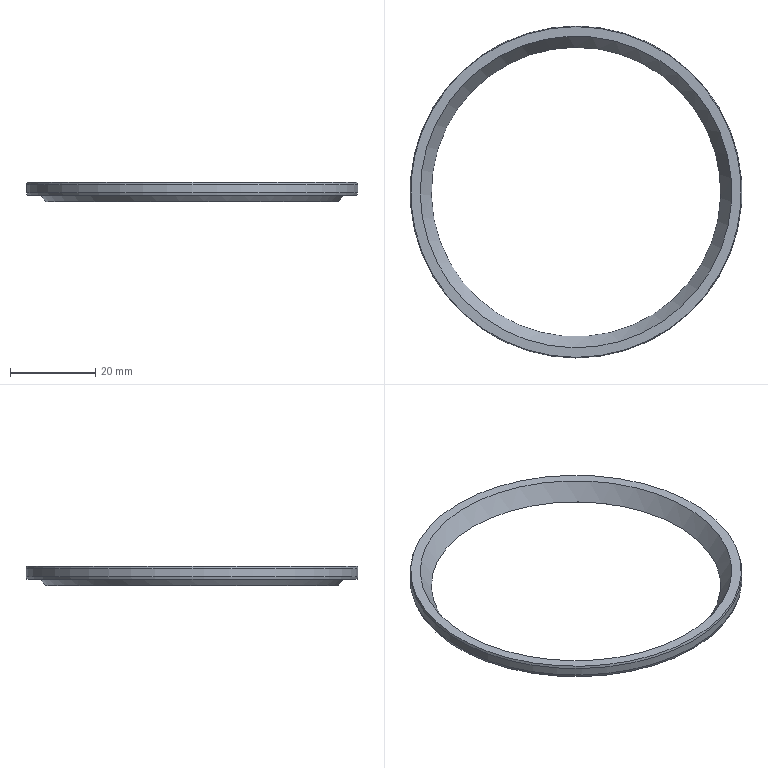Part | STEP file | 1 solid | 12 faces | box 78 x 78 x 4.5 mm | volume 2023 mm3 | cone 5 | plane 3 | cylinder 2 | torus 2 | commonest cylinder face diameters 75.4 x1 78 x1
STEP:
#1=CARTESIAN_POINT('',(33.645,-19.425,-11.25));
#2=VERTEX_POINT('',#1);
#3=CARTESIAN_POINT('',(0.,0.,-11.25));
#4=DIRECTION('',(0.,0.,1.));
#5=DIRECTION('',(0.866,0.5,0.));
#6=AXIS2_PLACEMENT_3D('',#3,#4,#5);
#7=CIRCLE('',#6,38.85);
#8=EDGE_CURVE('',#2,#2,#7,.T.);
#9=ORIENTED_EDGE('',*,*,#8,.T.);
#10=EDGE_LOOP('',(#9));
#11=FACE_BOUND('',#10,.T.);
#12=CARTESIAN_POINT('',(31.697,-18.3,-11.25));
#13=VERTEX_POINT('',#12);
#14=CARTESIAN_POINT('',(0.,0.,-11.25));
#15=DIRECTION('',(0.,0.,-1.));
#16=DIRECTION('',(0.,-1.,0.));
#17=AXIS2_PLACEMENT_3D('',#14,#15,#16);
#18=CIRCLE('',#17,36.6);
#19=EDGE_CURVE('',#13,#13,#18,.T.);
#20=ORIENTED_EDGE('',*,*,#19,.T.);
#21=EDGE_LOOP('',(#20));
#22=FACE_BOUND('',#21,.T.);
#23=CARTESIAN_POINT('',(0.,0.,-11.25));
#24=DIRECTION('',(0.,0.,-1.));
#25=DIRECTION('',(0.,-1.,0.));
#26=AXIS2_PLACEMENT_3D('',#23,#24,#25);
#27=PLANE('',#26);
#28=ADVANCED_FACE('',(#11,#22),#27,.F.);
#29=CARTESIAN_POINT('',(33.775,-19.5,-11.81));
#30=VERTEX_POINT('',#29);
#31=CARTESIAN_POINT('',(-33.775,19.5,-11.81));
#32=VERTEX_POINT('',#31);
#33=CARTESIAN_POINT('',(0.,0.,-11.81));
#34=DIRECTION('',(0.,0.,1.));
#35=DIRECTION('',(0.866,-0.5,0.));
#36=AXIS2_PLACEMENT_3D('',#33,#34,#35);
#37=CIRCLE('',#36,39.);
#38=EDGE_CURVE('',#30,#32,#37,.T.);
#39=ORIENTED_EDGE('',*,*,#38,.T.);
#40=CARTESIAN_POINT('',(0.,0.,-11.81));
#41=DIRECTION('',(0.,0.,1.));
#42=DIRECTION('',(-0.866,0.5,0.));
#43=AXIS2_PLACEMENT_3D('',#40,#41,#42);
#44=CIRCLE('',#43,39.);
#45=EDGE_CURVE('',#32,#30,#44,.T.);
#46=ORIENTED_EDGE('',*,*,#45,.T.);
#47=EDGE_LOOP('',(#39,#46));
#48=FACE_BOUND('',#47,.T.);
#49=ORIENTED_EDGE('',*,*,#8,.F.);
#50=EDGE_LOOP('',(#49));
#51=FACE_OUTER_BOUND('',#50,.T.);
#52=CARTESIAN_POINT('',(0.,0.,-11.53));
#53=DIRECTION('',(0.,0.,-1.));
#54=DIRECTION('',(0.866,-0.5,0.));
#55=AXIS2_PLACEMENT_3D('',#52,#53,#54);
#56=CONICAL_SURFACE('',#55,38.925,0.2617);
#57=ADVANCED_FACE('',(#48,#51),#56,.T.);
#58=ORIENTED_EDGE('',*,*,#45,.F.);
#59=ORIENTED_EDGE('',*,*,#38,.F.);
#60=EDGE_LOOP('',(#58,#59));
#61=FACE_BOUND('',#60,.T.);
#62=CARTESIAN_POINT('',(-33.775,19.5,-13.69));
#63=VERTEX_POINT('',#62);
#64=CARTESIAN_POINT('',(33.775,-19.5,-13.69));
#65=VERTEX_POINT('',#64);
#66=CARTESIAN_POINT('',(0.,0.,-13.69));
#67=DIRECTION('',(0.,0.,-1.));
#68=DIRECTION('',(-0.866,0.5,0.));
#69=AXIS2_PLACEMENT_3D('',#66,#67,#68);
#70=CIRCLE('',#69,39.);
#71=EDGE_CURVE('',#63,#65,#70,.T.);
#72=ORIENTED_EDGE('',*,*,#71,.F.);
#73=CARTESIAN_POINT('',(0.,0.,-13.69));
#74=DIRECTION('',(0.,0.,-1.));
#75=DIRECTION('',(0.866,-0.5,0.));
#76=AXIS2_PLACEMENT_3D('',#73,#74,#75);
#77=CIRCLE('',#76,39.);
#78=EDGE_CURVE('',#65,#63,#77,.T.);
#79=ORIENTED_EDGE('',*,*,#78,.F.);
#80=EDGE_LOOP('',(#72,#79));
#81=FACE_BOUND('',#80,.T.);
#82=CARTESIAN_POINT('',(0.,0.,-11.025));
#83=DIRECTION('',(0.,0.,1.));
#84=DIRECTION('',(0.866,-0.5,0.));
#85=AXIS2_PLACEMENT_3D('',#82,#83,#84);
#86=CYLINDRICAL_SURFACE('',#85,39.);
#87=ADVANCED_FACE('',(#61,#81),#86,.T.);
#88=ORIENTED_EDGE('',*,*,#78,.T.);
#89=ORIENTED_EDGE('',*,*,#71,.T.);
#90=EDGE_LOOP('',(#88,#89));
#91=FACE_BOUND('',#90,.T.);
#92=CARTESIAN_POINT('',(33.645,-19.425,-14.25));
#93=VERTEX_POINT('',#92);
#94=CARTESIAN_POINT('',(0.,0.,-14.25));
#95=DIRECTION('',(0.,0.,-1.));
#96=DIRECTION('',(0.,-1.,0.));
#97=AXIS2_PLACEMENT_3D('',#94,#95,#96);
#98=CIRCLE('',#97,38.85);
#99=EDGE_CURVE('',#93,#93,#98,.T.);
#100=ORIENTED_EDGE('',*,*,#99,.F.);
#101=EDGE_LOOP('',(#100));
#102=FACE_OUTER_BOUND('',#101,.T.);
#103=CARTESIAN_POINT('',(0.,0.,-13.97));
#104=DIRECTION('',(0.,0.,1.));
#105=DIRECTION('',(0.866,-0.5,0.));
#106=AXIS2_PLACEMENT_3D('',#103,#104,#105);
#107=CONICAL_SURFACE('',#106,38.925,0.2617);
#108=ADVANCED_FACE('',(#91,#102),#107,.T.);
#109=ORIENTED_EDGE('',*,*,#99,.T.);
#110=EDGE_LOOP('',(#109));
#111=FACE_BOUND('',#110,.T.);
#112=CARTESIAN_POINT('',(-32.649,18.85,-14.25));
#113=VERTEX_POINT('',#112);
#114=CARTESIAN_POINT('',(0.,0.,-14.25));
#115=DIRECTION('',(0.,0.,1.));
#116=DIRECTION('',(0.866,-0.5,0.));
#117=AXIS2_PLACEMENT_3D('',#114,#115,#116);
#118=CIRCLE('',#117,37.7);
#119=EDGE_CURVE('',#113,#113,#118,.T.);
#120=ORIENTED_EDGE('',*,*,#119,.T.);
#121=EDGE_LOOP('',(#120));
#122=FACE_BOUND('',#121,.T.);
#123=CARTESIAN_POINT('',(0.,0.,-14.25));
#124=DIRECTION('',(0.,0.,-1.));
#125=DIRECTION('',(0.,-1.,0.));
#126=AXIS2_PLACEMENT_3D('',#123,#124,#125);
#127=PLANE('',#126);
#128=ADVANCED_FACE('',(#111,#122),#127,.T.);
#129=CARTESIAN_POINT('',(-32.649,18.85,-13.05));
#130=VERTEX_POINT('',#129);
#131=CARTESIAN_POINT('',(-32.649,18.85,-13.05));
#132=CARTESIAN_POINT('',(-32.254,19.534,-13.05));
#133=CARTESIAN_POINT('',(-31.422,20.877,-13.05));
#134=CARTESIAN_POINT('',(-30.048,22.809,-13.05));
#135=CARTESIAN_POINT('',(-28.557,24.651,-13.05));
#136=CARTESIAN_POINT('',(-26.952,26.396,-13.05));
#137=CARTESIAN_POINT('',(-25.241,28.036,-13.05));
#138=CARTESIAN_POINT('',(-23.431,29.566,-13.05));
#139=CARTESIAN_POINT('',(-21.528,30.979,-13.05));
#140=CARTESIAN_POINT('',(-19.54,32.27,-13.05));
#141=CARTESIAN_POINT('',(-17.475,33.433,-13.05));
#142=CARTESIAN_POINT('',(-15.341,34.465,-13.05));
#143=CARTESIAN_POINT('',(-13.146,35.36,-13.05));
#144=CARTESIAN_POINT('',(-10.899,36.116,-13.05));
#145=CARTESIAN_POINT('',(-8.61,36.729,-13.05));
#146=CARTESIAN_POINT('',(-6.286,37.197,-13.05));
#147=CARTESIAN_POINT('',(-3.938,37.519,-13.05));
#148=CARTESIAN_POINT('',(-1.574,37.692,-13.05));
#149=CARTESIAN_POINT('',(0.7965,37.716,-13.05));
#150=CARTESIAN_POINT('',(3.163,37.592,-13.05));
#151=CARTESIAN_POINT('',(5.518,37.319,-13.05));
#152=CARTESIAN_POINT('',(7.851,36.899,-13.05));
#153=CARTESIAN_POINT('',(10.153,36.333,-13.05));
#154=CARTESIAN_POINT('',(12.414,35.624,-13.05));
#155=CARTESIAN_POINT('',(14.627,34.774,-13.05));
#156=CARTESIAN_POINT('',(16.782,33.787,-13.05));
#157=CARTESIAN_POINT('',(18.871,32.666,-13.05));
#158=CARTESIAN_POINT('',(20.885,31.416,-13.05));
#159=CARTESIAN_POINT('',(22.817,30.043,-13.05));
#160=CARTESIAN_POINT('',(24.658,28.551,-13.05));
#161=CARTESIAN_POINT('',(26.402,26.946,-13.05));
#162=CARTESIAN_POINT('',(28.043,25.234,-13.05));
#163=CARTESIAN_POINT('',(29.572,23.424,-13.05));
#164=CARTESIAN_POINT('',(30.985,21.52,-13.05));
#165=CARTESIAN_POINT('',(32.275,19.532,-13.05));
#166=CARTESIAN_POINT('',(33.438,17.466,-13.05));
#167=CARTESIAN_POINT('',(34.469,15.332,-13.05));
#168=CARTESIAN_POINT('',(35.364,13.137,-13.05));
#169=CARTESIAN_POINT('',(36.119,10.89,-13.05));
#170=CARTESIAN_POINT('',(36.731,8.601,-13.05));
#171=CARTESIAN_POINT('',(37.199,6.277,-13.05));
#172=CARTESIAN_POINT('',(37.52,3.928,-13.05));
#173=CARTESIAN_POINT('',(37.692,1.564,-13.05));
#174=CARTESIAN_POINT('',(37.716,-0.8059,-13.05));
#175=CARTESIAN_POINT('',(37.591,-3.173,-13.05));
#176=CARTESIAN_POINT('',(37.318,-5.527,-13.05));
#177=CARTESIAN_POINT('',(36.897,-7.86,-13.05));
#178=CARTESIAN_POINT('',(36.33,-10.162,-13.05));
#179=CARTESIAN_POINT('',(35.621,-12.423,-13.05));
#180=CARTESIAN_POINT('',(34.77,-14.636,-13.05));
#181=CARTESIAN_POINT('',(33.785,-16.785,-13.05));
#182=CARTESIAN_POINT('',(33.041,-18.172,-13.05));
#183=CARTESIAN_POINT('',(32.649,-18.85,-13.05));
#184=CARTESIAN_POINT('',(32.254,-19.534,-13.05));
#185=CARTESIAN_POINT('',(31.422,-20.877,-13.05));
#186=CARTESIAN_POINT('',(30.048,-22.809,-13.05));
#187=CARTESIAN_POINT('',(28.557,-24.651,-13.05));
#188=CARTESIAN_POINT('',(26.952,-26.396,-13.05));
#189=CARTESIAN_POINT('',(25.241,-28.036,-13.05));
#190=CARTESIAN_POINT('',(23.431,-29.566,-13.05));
#191=CARTESIAN_POINT('',(21.528,-30.979,-13.05));
#192=CARTESIAN_POINT('',(19.54,-32.27,-13.05));
#193=CARTESIAN_POINT('',(17.475,-33.433,-13.05));
#194=CARTESIAN_POINT('',(15.341,-34.465,-13.05));
#195=CARTESIAN_POINT('',(13.146,-35.36,-13.05));
#196=CARTESIAN_POINT('',(10.899,-36.116,-13.05));
#197=CARTESIAN_POINT('',(8.61,-36.729,-13.05));
#198=CARTESIAN_POINT('',(6.286,-37.197,-13.05));
#199=CARTESIAN_POINT('',(3.938,-37.519,-13.05));
#200=CARTESIAN_POINT('',(1.574,-37.692,-13.05));
#201=CARTESIAN_POINT('',(-0.7965,-37.716,-13.05));
#202=CARTESIAN_POINT('',(-3.163,-37.592,-13.05));
#203=CARTESIAN_POINT('',(-5.518,-37.319,-13.05));
#204=CARTESIAN_POINT('',(-7.851,-36.899,-13.05));
#205=CARTESIAN_POINT('',(-10.153,-36.333,-13.05));
#206=CARTESIAN_POINT('',(-12.414,-35.624,-13.05));
#207=CARTESIAN_POINT('',(-14.627,-34.774,-13.05));
#208=CARTESIAN_POINT('',(-16.782,-33.787,-13.05));
#209=CARTESIAN_POINT('',(-18.871,-32.666,-13.05));
#210=CARTESIAN_POINT('',(-20.885,-31.416,-13.05));
#211=CARTESIAN_POINT('',(-22.817,-30.043,-13.05));
#212=CARTESIAN_POINT('',(-24.658,-28.551,-13.05));
#213=CARTESIAN_POINT('',(-26.402,-26.946,-13.05));
#214=CARTESIAN_POINT('',(-28.043,-25.234,-13.05));
#215=CARTESIAN_POINT('',(-29.572,-23.424,-13.05));
#216=CARTESIAN_POINT('',(-30.985,-21.52,-13.05));
#217=CARTESIAN_POINT('',(-32.275,-19.532,-13.05));
#218=CARTESIAN_POINT('',(-33.438,-17.466,-13.05));
#219=CARTESIAN_POINT('',(-34.469,-15.332,-13.05));
#220=CARTESIAN_POINT('',(-35.364,-13.137,-13.05));
#221=CARTESIAN_POINT('',(-36.119,-10.89,-13.05));
#222=CARTESIAN_POINT('',(-36.731,-8.601,-13.05));
#223=CARTESIAN_POINT('',(-37.199,-6.277,-13.05));
#224=CARTESIAN_POINT('',(-37.52,-3.928,-13.05));
#225=CARTESIAN_POINT('',(-37.692,-1.564,-13.05));
#226=CARTESIAN_POINT('',(-37.716,0.8059,-13.05));
#227=CARTESIAN_POINT('',(-37.591,3.173,-13.05));
#228=CARTESIAN_POINT('',(-37.318,5.527,-13.05));
#229=CARTESIAN_POINT('',(-36.897,7.86,-13.05));
#230=CARTESIAN_POINT('',(-36.33,10.162,-13.05));
#231=CARTESIAN_POINT('',(-35.621,12.423,-13.05));
#232=CARTESIAN_POINT('',(-34.77,14.636,-13.05));
#233=CARTESIAN_POINT('',(-33.785,16.785,-13.05));
#234=CARTESIAN_POINT('',(-33.041,18.172,-13.05));
#235=CARTESIAN_POINT('',(-32.649,18.85,-13.05));
#236=B_SPLINE_CURVE_WITH_KNOTS('',3,(#131,#132,#133,#134,#135,#136,#137,#138,#139,#140,#141,#142,#143,#144,#145,#146,#147,#148,#149,#150,#151,#152,#153,#154,#155,#156,#157,#158,#159,#160,#161,#162,#163,#164,#165,#166,#167,#168,#169,#170,#171,#172,#173,#174,#175,#176,#177,#178,#179,#180,#181,#182,#183,#184,#185,#186,#187,#188,#189,#190,#191,#192,#193,#194,#195,#196,#197,#198,#199,#200,#201,#202,#203,#204,#205,#206,#207,#208,#209,#210,#211,#212,#213,#214,#215,#216,#217,#218,#219,#220,#221,#222,#223,#224,#225,#226,#227,#228,#229,#230,#231,#232,#233,#234,#235),.UNSPECIFIED.,.T.,.F.,(4,1,1,1,1,1,1,1,1,1,1,1,1,1,1,1,1,1,1,1,1,1,1,1,1,1,1,1,1,1,1,1,1,1,1,1,1,1,1,1,1,1,1,1,1,1,1,1,1,1,3,1,1,1,1,1,1,1,1,1,1,1,1,1,1,1,1,1,1,1,1,1,1,1,1,1,1,1,1,1,1,1,1,1,1,1,1,1,1,1,1,1,1,1,1,1,1,1,1,1,4),(0.,0.01,0.02,0.03,0.04001,0.05001,0.06001,0.07001,0.08001,0.09001,0.1,0.11,0.12,0.13,0.14,0.15,0.16,0.17,0.18,0.19,0.2,0.21,0.22,0.23,0.24,0.25,0.26,0.27,0.28,0.29,0.3,0.31,0.3201,0.3301,0.3401,0.3501,0.3601,0.3701,0.3801,0.3901,0.4001,0.4101,0.4201,0.4301,0.4401,0.4501,0.4601,0.4701,0.4801,0.4901,0.5,0.51,0.52,0.53,0.54,0.55,0.56,0.57,0.58,0.59,0.6,0.61,0.62,0.63,0.64,0.65,0.66,0.67,0.68,0.69,0.7,0.71,0.72,0.73,0.74,0.75,0.76,0.77,0.78,0.79,0.8,0.81,0.8201,0.8301,0.8401,0.8501,0.8601,0.8701,0.8801,0.8901,0.9001,0.9101,0.9201,0.9301,0.9401,0.9501,0.9601,0.9701,0.9801,0.9901,1.),.UNSPECIFIED.);
#237=EDGE_CURVE('',#130,#130,#236,.T.);
#238=ORIENTED_EDGE('',*,*,#237,.F.);
#239=EDGE_LOOP('',(#238));
#240=FACE_OUTER_BOUND('',#239,.T.);
#241=ORIENTED_EDGE('',*,*,#119,.F.);
#242=EDGE_LOOP('',(#241));
#243=FACE_OUTER_BOUND('',#242,.T.);
#244=CARTESIAN_POINT('',(0.,0.,-11.025));
#245=DIRECTION('',(0.,0.,1.));
#246=DIRECTION('',(0.866,-0.5,0.));
#247=AXIS2_PLACEMENT_3D('',#244,#245,#246);
#248=CYLINDRICAL_SURFACE('',#247,37.7);
#249=ADVANCED_FACE('',(#240,#243),#248,.F.);
#250=CARTESIAN_POINT('',(-32.389,18.7,-12.75));
#251=VERTEX_POINT('',#250);
#252=CARTESIAN_POINT('',(0.,0.,-12.75));
#253=DIRECTION('',(0.,0.,-1.));
#254=DIRECTION('',(0.866,-0.5,0.));
#255=AXIS2_PLACEMENT_3D('',#252,#253,#254);
#256=CIRCLE('',#255,37.4);
#257=EDGE_CURVE('',#251,#251,#256,.T.);
#258=ORIENTED_EDGE('',*,*,#257,.F.);
#259=EDGE_LOOP('',(#258));
#260=FACE_OUTER_BOUND('',#259,.T.);
#261=ORIENTED_EDGE('',*,*,#237,.T.);
#262=EDGE_LOOP('',(#261));
#263=FACE_OUTER_BOUND('',#262,.T.);
#264=CARTESIAN_POINT('',(0.,0.,-13.05));
#265=DIRECTION('',(0.,0.,-1.));
#266=DIRECTION('',(0.866,-0.5,0.));
#267=AXIS2_PLACEMENT_3D('',#264,#265,#266);
#268=TOROIDAL_SURFACE('',#267,37.4,0.3);
#269=ADVANCED_FACE('',(#260,#263),#268,.F.);
#270=ORIENTED_EDGE('',*,*,#257,.T.);
#271=EDGE_LOOP('',(#270));
#272=FACE_BOUND('',#271,.T.);
#273=CARTESIAN_POINT('',(-32.008,18.48,-12.75));
#274=VERTEX_POINT('',#273);
#275=CARTESIAN_POINT('',(0.,0.,-12.75));
#276=DIRECTION('',(0.,0.,1.));
#277=DIRECTION('',(0.866,-0.5,0.));
#278=AXIS2_PLACEMENT_3D('',#275,#276,#277);
#279=CIRCLE('',#278,36.959);
#280=EDGE_CURVE('',#274,#274,#279,.T.);
#281=ORIENTED_EDGE('',*,*,#280,.T.);
#282=EDGE_LOOP('',(#281));
#283=FACE_BOUND('',#282,.T.);
#284=CARTESIAN_POINT('',(0.,0.,-12.75));
#285=DIRECTION('',(0.,0.,-1.));
#286=DIRECTION('',(0.,-1.,0.));
#287=AXIS2_PLACEMENT_3D('',#284,#285,#286);
#288=PLANE('',#287);
#289=ADVANCED_FACE('',(#272,#283),#288,.T.);
#290=CARTESIAN_POINT('',(31.804,-18.362,-12.863));
#291=VERTEX_POINT('',#290);
#292=CARTESIAN_POINT('',(-31.804,18.362,-12.863));
#293=VERTEX_POINT('',#292);
#294=CARTESIAN_POINT('',(0.,0.,-12.863));
#295=DIRECTION('',(0.,0.,1.));
#296=DIRECTION('',(0.866,-0.5,0.));
#297=AXIS2_PLACEMENT_3D('',#294,#295,#296);
#298=CIRCLE('',#297,36.725);
#299=EDGE_CURVE('',#291,#293,#298,.T.);
#300=ORIENTED_EDGE('',*,*,#299,.T.);
#301=CARTESIAN_POINT('',(0.,0.,-12.863));
#302=DIRECTION('',(0.,0.,1.));
#303=DIRECTION('',(-0.866,0.5,0.));
#304=AXIS2_PLACEMENT_3D('',#301,#302,#303);
#305=CIRCLE('',#304,36.725);
#306=EDGE_CURVE('',#293,#291,#305,.T.);
#307=ORIENTED_EDGE('',*,*,#306,.T.);
#308=EDGE_LOOP('',(#300,#307));
#309=FACE_BOUND('',#308,.T.);
#310=ORIENTED_EDGE('',*,*,#280,.F.);
#311=EDGE_LOOP('',(#310));
#312=FACE_OUTER_BOUND('',#311,.T.);
#313=CARTESIAN_POINT('',(0.,0.,-13.05));
#314=DIRECTION('',(0.,0.,-1.));
#315=DIRECTION('',(0.866,-0.5,0.));
#316=AXIS2_PLACEMENT_3D('',#313,#314,#315);
#317=TOROIDAL_SURFACE('',#316,36.959,0.3);
#318=ADVANCED_FACE('',(#309,#312),#317,.F.);
#319=ORIENTED_EDGE('',*,*,#306,.F.);
#320=ORIENTED_EDGE('',*,*,#299,.F.);
#321=EDGE_LOOP('',(#319,#320));
#322=FACE_BOUND('',#321,.T.);
#323=CARTESIAN_POINT('',(29.814,-17.213,-15.75));
#324=VERTEX_POINT('',#323);
#325=CARTESIAN_POINT('',(29.814,-17.213,-15.75));
#326=CARTESIAN_POINT('',(29.453,-17.838,-15.75));
#327=CARTESIAN_POINT('',(28.693,-19.064,-15.75));
#328=CARTESIAN_POINT('',(27.439,-20.828,-15.75));
#329=CARTESIAN_POINT('',(26.077,-22.51,-15.75));
#330=CARTESIAN_POINT('',(24.612,-24.104,-15.75));
#331=CARTESIAN_POINT('',(23.05,-25.602,-15.75));
#332=CARTESIAN_POINT('',(21.396,-26.999,-15.75));
#333=CARTESIAN_POINT('',(19.658,-28.289,-15.75));
#334=CARTESIAN_POINT('',(17.843,-29.468,-15.75));
#335=CARTESIAN_POINT('',(15.957,-30.53,-15.75));
#336=CARTESIAN_POINT('',(14.008,-31.472,-15.75));
#337=CARTESIAN_POINT('',(12.004,-32.29,-15.75));
#338=CARTESIAN_POINT('',(9.953,-32.98,-15.75));
#339=CARTESIAN_POINT('',(7.862,-33.54,-15.75));
#340=CARTESIAN_POINT('',(5.74,-33.967,-15.75));
#341=CARTESIAN_POINT('',(3.596,-34.261,-15.75));
#342=CARTESIAN_POINT('',(1.437,-34.419,-15.75));
#343=CARTESIAN_POINT('',(-0.7273,-34.441,-15.75));
#344=CARTESIAN_POINT('',(-2.889,-34.328,-15.75));
#345=CARTESIAN_POINT('',(-5.039,-34.078,-15.75));
#346=CARTESIAN_POINT('',(-7.169,-33.695,-15.75));
#347=CARTESIAN_POINT('',(-9.271,-33.178,-15.75));
#348=CARTESIAN_POINT('',(-11.336,-32.53,-15.75));
#349=CARTESIAN_POINT('',(-13.357,-31.754,-15.75));
#350=CARTESIAN_POINT('',(-15.325,-30.853,-15.75));
#351=CARTESIAN_POINT('',(-17.232,-29.829,-15.75));
#352=CARTESIAN_POINT('',(-19.071,-28.688,-15.75));
#353=CARTESIAN_POINT('',(-20.835,-27.434,-15.75));
#354=CARTESIAN_POINT('',(-22.517,-26.071,-15.75));
#355=CARTESIAN_POINT('',(-24.11,-24.606,-15.75));
#356=CARTESIAN_POINT('',(-25.607,-23.043,-15.75));
#357=CARTESIAN_POINT('',(-27.004,-21.389,-15.75));
#358=CARTESIAN_POINT('',(-28.294,-19.651,-15.75));
#359=CARTESIAN_POINT('',(-29.472,-17.836,-15.75));
#360=CARTESIAN_POINT('',(-30.534,-15.95,-15.75));
#361=CARTESIAN_POINT('',(-31.476,-14.001,-15.75));
#362=CARTESIAN_POINT('',(-32.293,-11.996,-15.75));
#363=CARTESIAN_POINT('',(-32.982,-9.945,-15.75));
#364=CARTESIAN_POINT('',(-33.542,-7.854,-15.75));
#365=CARTESIAN_POINT('',(-33.969,-5.732,-15.75));
#366=CARTESIAN_POINT('',(-34.262,-3.587,-15.75));
#367=CARTESIAN_POINT('',(-34.419,-1.428,-15.75));
#368=CARTESIAN_POINT('',(-34.441,0.7359,-15.75));
#369=CARTESIAN_POINT('',(-34.327,2.897,-15.75));
#370=CARTESIAN_POINT('',(-34.077,5.047,-15.75));
#371=CARTESIAN_POINT('',(-33.693,7.177,-15.75));
#372=CARTESIAN_POINT('',(-33.176,9.279,-15.75));
#373=CARTESIAN_POINT('',(-32.527,11.344,-15.75));
#374=CARTESIAN_POINT('',(-31.751,13.365,-15.75));
#375=CARTESIAN_POINT('',(-30.851,15.327,-15.75));
#376=CARTESIAN_POINT('',(-30.172,16.594,-15.75));
#377=CARTESIAN_POINT('',(-29.814,17.213,-15.75));
#378=CARTESIAN_POINT('',(-29.453,17.838,-15.75));
#379=CARTESIAN_POINT('',(-28.693,19.064,-15.75));
#380=CARTESIAN_POINT('',(-27.439,20.828,-15.75));
#381=CARTESIAN_POINT('',(-26.077,22.51,-15.75));
#382=CARTESIAN_POINT('',(-24.612,24.104,-15.75));
#383=CARTESIAN_POINT('',(-23.05,25.602,-15.75));
#384=CARTESIAN_POINT('',(-21.396,26.999,-15.75));
#385=CARTESIAN_POINT('',(-19.658,28.289,-15.75));
#386=CARTESIAN_POINT('',(-17.843,29.468,-15.75));
#387=CARTESIAN_POINT('',(-15.957,30.53,-15.75));
#388=CARTESIAN_POINT('',(-14.008,31.472,-15.75));
#389=CARTESIAN_POINT('',(-12.004,32.29,-15.75));
#390=CARTESIAN_POINT('',(-9.953,32.98,-15.75));
#391=CARTESIAN_POINT('',(-7.862,33.54,-15.75));
#392=CARTESIAN_POINT('',(-5.74,33.967,-15.75));
#393=CARTESIAN_POINT('',(-3.596,34.261,-15.75));
#394=CARTESIAN_POINT('',(-1.437,34.419,-15.75));
#395=CARTESIAN_POINT('',(0.7273,34.441,-15.75));
#396=CARTESIAN_POINT('',(2.889,34.328,-15.75));
#397=CARTESIAN_POINT('',(5.039,34.078,-15.75));
#398=CARTESIAN_POINT('',(7.169,33.695,-15.75));
#399=CARTESIAN_POINT('',(9.271,33.178,-15.75));
#400=CARTESIAN_POINT('',(11.336,32.53,-15.75));
#401=CARTESIAN_POINT('',(13.357,31.754,-15.75));
#402=CARTESIAN_POINT('',(15.325,30.853,-15.75));
#403=CARTESIAN_POINT('',(17.232,29.829,-15.75));
#404=CARTESIAN_POINT('',(19.071,28.688,-15.75));
#405=CARTESIAN_POINT('',(20.835,27.434,-15.75));
#406=CARTESIAN_POINT('',(22.517,26.071,-15.75));
#407=CARTESIAN_POINT('',(24.11,24.606,-15.75));
#408=CARTESIAN_POINT('',(25.607,23.043,-15.75));
#409=CARTESIAN_POINT('',(27.004,21.389,-15.75));
#410=CARTESIAN_POINT('',(28.294,19.651,-15.75));
#411=CARTESIAN_POINT('',(29.472,17.836,-15.75));
#412=CARTESIAN_POINT('',(30.534,15.95,-15.75));
#413=CARTESIAN_POINT('',(31.476,14.001,-15.75));
#414=CARTESIAN_POINT('',(32.293,11.996,-15.75));
#415=CARTESIAN_POINT('',(32.982,9.945,-15.75));
#416=CARTESIAN_POINT('',(33.542,7.854,-15.75));
#417=CARTESIAN_POINT('',(33.969,5.732,-15.75));
#418=CARTESIAN_POINT('',(34.262,3.587,-15.75));
#419=CARTESIAN_POINT('',(34.419,1.428,-15.75));
#420=CARTESIAN_POINT('',(34.441,-0.7359,-15.75));
#421=CARTESIAN_POINT('',(34.327,-2.897,-15.75));
#422=CARTESIAN_POINT('',(34.077,-5.047,-15.75));
#423=CARTESIAN_POINT('',(33.693,-7.177,-15.75));
#424=CARTESIAN_POINT('',(33.176,-9.279,-15.75));
#425=CARTESIAN_POINT('',(32.527,-11.344,-15.75));
#426=CARTESIAN_POINT('',(31.751,-13.365,-15.75));
#427=CARTESIAN_POINT('',(30.851,-15.327,-15.75));
#428=CARTESIAN_POINT('',(30.172,-16.594,-15.75));
#429=CARTESIAN_POINT('',(29.814,-17.213,-15.75));
#430=B_SPLINE_CURVE_WITH_KNOTS('',3,(#325,#326,#327,#328,#329,#330,#331,#332,#333,#334,#335,#336,#337,#338,#339,#340,#341,#342,#343,#344,#345,#346,#347,#348,#349,#350,#351,#352,#353,#354,#355,#356,#357,#358,#359,#360,#361,#362,#363,#364,#365,#366,#367,#368,#369,#370,#371,#372,#373,#374,#375,#376,#377,#378,#379,#380,#381,#382,#383,#384,#385,#386,#387,#388,#389,#390,#391,#392,#393,#394,#395,#396,#397,#398,#399,#400,#401,#402,#403,#404,#405,#406,#407,#408,#409,#410,#411,#412,#413,#414,#415,#416,#417,#418,#419,#420,#421,#422,#423,#424,#425,#426,#427,#428,#429),.UNSPECIFIED.,.T.,.F.,(4,1,1,1,1,1,1,1,1,1,1,1,1,1,1,1,1,1,1,1,1,1,1,1,1,1,1,1,1,1,1,1,1,1,1,1,1,1,1,1,1,1,1,1,1,1,1,1,1,1,3,1,1,1,1,1,1,1,1,1,1,1,1,1,1,1,1,1,1,1,1,1,1,1,1,1,1,1,1,1,1,1,1,1,1,1,1,1,1,1,1,1,1,1,1,1,1,1,1,1,4),(0.,0.01,0.02,0.03,0.04001,0.05001,0.06001,0.07001,0.08001,0.09001,0.1,0.11,0.12,0.13,0.14,0.15,0.16,0.17,0.18,0.19,0.2,0.21,0.22,0.23,0.24,0.25,0.26,0.27,0.28,0.29,0.3,0.31,0.3201,0.3301,0.3401,0.3501,0.3601,0.3701,0.3801,0.3901,0.4001,0.4101,0.4201,0.4301,0.4401,0.4501,0.4601,0.4701,0.4801,0.4901,0.5,0.51,0.52,0.53,0.54,0.55,0.56,0.57,0.58,0.59,0.6,0.61,0.62,0.63,0.64,0.65,0.66,0.67,0.68,0.69,0.7,0.71,0.72,0.73,0.74,0.75,0.76,0.77,0.78,0.79,0.8,0.81,0.8201,0.8301,0.8401,0.8501,0.8601,0.8701,0.8801,0.8901,0.9001,0.9101,0.9201,0.9301,0.9401,0.9501,0.9601,0.9701,0.9801,0.9901,1.),.UNSPECIFIED.);
#431=EDGE_CURVE('',#324,#324,#430,.T.);
#432=ORIENTED_EDGE('',*,*,#431,.F.);
#433=EDGE_LOOP('',(#432));
#434=FACE_OUTER_BOUND('',#433,.T.);
#435=CARTESIAN_POINT('',(0.,0.,-14.307));
#436=DIRECTION('',(0.,0.,1.));
#437=DIRECTION('',(0.866,-0.5,0.));
#438=AXIS2_PLACEMENT_3D('',#435,#436,#437);
#439=CONICAL_SURFACE('',#438,35.575,0.6724);
#440=ADVANCED_FACE('',(#322,#434),#439,.T.);
#441=ORIENTED_EDGE('',*,*,#431,.T.);
#442=EDGE_LOOP('',(#441));
#443=FACE_OUTER_BOUND('',#442,.T.);
#444=CARTESIAN_POINT('',(29.445,-17.,-15.489));
#445=VERTEX_POINT('',#444);
#446=CARTESIAN_POINT('',(29.445,-17.,-15.489));
#447=CARTESIAN_POINT('',(29.089,-17.617,-15.489));
#448=CARTESIAN_POINT('',(28.338,-18.828,-15.489));
#449=CARTESIAN_POINT('',(27.099,-20.57,-15.489));
#450=CARTESIAN_POINT('',(25.754,-22.232,-15.489));
#451=CARTESIAN_POINT('',(24.307,-23.805,-15.489));
#452=CARTESIAN_POINT('',(22.764,-25.285,-15.489));
#453=CARTESIAN_POINT('',(21.131,-26.664,-15.489));
#454=CARTESIAN_POINT('',(19.415,-27.939,-15.489));
#455=CARTESIAN_POINT('',(17.622,-29.103,-15.489));
#456=CARTESIAN_POINT('',(15.76,-30.152,-15.489));
#457=CARTESIAN_POINT('',(13.835,-31.082,-15.489));
#458=CARTESIAN_POINT('',(11.856,-31.89,-15.489));
#459=CARTESIAN_POINT('',(9.83,-32.571,-15.489));
#460=CARTESIAN_POINT('',(7.765,-33.124,-15.489));
#461=CARTESIAN_POINT('',(5.669,-33.547,-15.489));
#462=CARTESIAN_POINT('',(3.551,-33.837,-15.489));
#463=CARTESIAN_POINT('',(1.419,-33.993,-15.489));
#464=CARTESIAN_POINT('',(-0.7183,-34.015,-15.489));
#465=CARTESIAN_POINT('',(-2.853,-33.903,-15.489));
#466=CARTESIAN_POINT('',(-4.976,-33.656,-15.489));
#467=CARTESIAN_POINT('',(-7.08,-33.277,-15.489));
#468=CARTESIAN_POINT('',(-9.156,-32.767,-15.489));
#469=CARTESIAN_POINT('',(-11.196,-32.127,-15.489));
#470=CARTESIAN_POINT('',(-13.191,-31.361,-15.489));
#471=CARTESIAN_POINT('',(-15.135,-30.471,-15.489));
#472=CARTESIAN_POINT('',(-17.019,-29.46,-15.489));
#473=CARTESIAN_POINT('',(-18.835,-28.333,-15.489));
#474=CARTESIAN_POINT('',(-20.577,-27.094,-15.489));
#475=CARTESIAN_POINT('',(-22.238,-25.749,-15.489));
#476=CARTESIAN_POINT('',(-23.811,-24.301,-15.489));
#477=CARTESIAN_POINT('',(-25.29,-22.758,-15.489));
#478=CARTESIAN_POINT('',(-26.67,-21.125,-15.489));
#479=CARTESIAN_POINT('',(-27.944,-19.408,-15.489));
#480=CARTESIAN_POINT('',(-29.107,-17.615,-15.489));
#481=CARTESIAN_POINT('',(-30.156,-15.752,-15.489));
#482=CARTESIAN_POINT('',(-31.086,-13.827,-15.489));
#483=CARTESIAN_POINT('',(-31.893,-11.848,-15.489));
#484=CARTESIAN_POINT('',(-32.574,-9.821,-15.489));
#485=CARTESIAN_POINT('',(-33.126,-7.756,-15.489));
#486=CARTESIAN_POINT('',(-33.548,-5.661,-15.489));
#487=CARTESIAN_POINT('',(-33.837,-3.543,-15.489));
#488=CARTESIAN_POINT('',(-33.993,-1.411,-15.489));
#489=CARTESIAN_POINT('',(-34.015,0.7268,-15.489));
#490=CARTESIAN_POINT('',(-33.902,2.861,-15.489));
#491=CARTESIAN_POINT('',(-33.655,4.985,-15.489));
#492=CARTESIAN_POINT('',(-33.276,7.089,-15.489));
#493=CARTESIAN_POINT('',(-32.765,9.164,-15.489));
#494=CARTESIAN_POINT('',(-32.125,11.204,-15.489));
#495=CARTESIAN_POINT('',(-31.358,13.199,-15.489));
#496=CARTESIAN_POINT('',(-30.469,15.137,-15.489));
#497=CARTESIAN_POINT('',(-29.798,16.388,-15.489));
#498=CARTESIAN_POINT('',(-29.445,17.,-15.489));
#499=CARTESIAN_POINT('',(-29.089,17.617,-15.489));
#500=CARTESIAN_POINT('',(-28.338,18.828,-15.489));
#501=CARTESIAN_POINT('',(-27.099,20.57,-15.489));
#502=CARTESIAN_POINT('',(-25.754,22.232,-15.489));
#503=CARTESIAN_POINT('',(-24.307,23.805,-15.489));
#504=CARTESIAN_POINT('',(-22.764,25.285,-15.489));
#505=CARTESIAN_POINT('',(-21.131,26.664,-15.489));
#506=CARTESIAN_POINT('',(-19.415,27.939,-15.489));
#507=CARTESIAN_POINT('',(-17.622,29.103,-15.489));
#508=CARTESIAN_POINT('',(-15.76,30.152,-15.489));
#509=CARTESIAN_POINT('',(-13.835,31.082,-15.489));
#510=CARTESIAN_POINT('',(-11.856,31.89,-15.489));
#511=CARTESIAN_POINT('',(-9.83,32.571,-15.489));
#512=CARTESIAN_POINT('',(-7.765,33.124,-15.489));
#513=CARTESIAN_POINT('',(-5.669,33.547,-15.489));
#514=CARTESIAN_POINT('',(-3.551,33.837,-15.489));
#515=CARTESIAN_POINT('',(-1.419,33.993,-15.489));
#516=CARTESIAN_POINT('',(0.7183,34.015,-15.489));
#517=CARTESIAN_POINT('',(2.853,33.903,-15.489));
#518=CARTESIAN_POINT('',(4.976,33.656,-15.489));
#519=CARTESIAN_POINT('',(7.08,33.277,-15.489));
#520=CARTESIAN_POINT('',(9.156,32.767,-15.489));
#521=CARTESIAN_POINT('',(11.196,32.127,-15.489));
#522=CARTESIAN_POINT('',(13.191,31.361,-15.489));
#523=CARTESIAN_POINT('',(15.135,30.471,-15.489));
#524=CARTESIAN_POINT('',(17.019,29.46,-15.489));
#525=CARTESIAN_POINT('',(18.835,28.333,-15.489));
#526=CARTESIAN_POINT('',(20.577,27.094,-15.489));
#527=CARTESIAN_POINT('',(22.238,25.749,-15.489));
#528=CARTESIAN_POINT('',(23.811,24.301,-15.489));
#529=CARTESIAN_POINT('',(25.29,22.758,-15.489));
#530=CARTESIAN_POINT('',(26.67,21.125,-15.489));
#531=CARTESIAN_POINT('',(27.944,19.408,-15.489));
#532=CARTESIAN_POINT('',(29.107,17.615,-15.489));
#533=CARTESIAN_POINT('',(30.156,15.752,-15.489));
#534=CARTESIAN_POINT('',(31.086,13.827,-15.489));
#535=CARTESIAN_POINT('',(31.893,11.848,-15.489));
#536=CARTESIAN_POINT('',(32.574,9.821,-15.489));
#537=CARTESIAN_POINT('',(33.126,7.756,-15.489));
#538=CARTESIAN_POINT('',(33.548,5.661,-15.489));
#539=CARTESIAN_POINT('',(33.837,3.543,-15.489));
#540=CARTESIAN_POINT('',(33.993,1.411,-15.489));
#541=CARTESIAN_POINT('',(34.015,-0.7268,-15.489));
#542=CARTESIAN_POINT('',(33.902,-2.861,-15.489));
#543=CARTESIAN_POINT('',(33.655,-4.985,-15.489));
#544=CARTESIAN_POINT('',(33.276,-7.089,-15.489));
#545=CARTESIAN_POINT('',(32.765,-9.164,-15.489));
#546=CARTESIAN_POINT('',(32.125,-11.204,-15.489));
#547=CARTESIAN_POINT('',(31.358,-13.199,-15.489));
#548=CARTESIAN_POINT('',(30.469,-15.137,-15.489));
#549=CARTESIAN_POINT('',(29.798,-16.388,-15.489));
#550=CARTESIAN_POINT('',(29.445,-17.,-15.489));
#551=B_SPLINE_CURVE_WITH_KNOTS('',3,(#446,#447,#448,#449,#450,#451,#452,#453,#454,#455,#456,#457,#458,#459,#460,#461,#462,#463,#464,#465,#466,#467,#468,#469,#470,#471,#472,#473,#474,#475,#476,#477,#478,#479,#480,#481,#482,#483,#484,#485,#486,#487,#488,#489,#490,#491,#492,#493,#494,#495,#496,#497,#498,#499,#500,#501,#502,#503,#504,#505,#506,#507,#508,#509,#510,#511,#512,#513,#514,#515,#516,#517,#518,#519,#520,#521,#522,#523,#524,#525,#526,#527,#528,#529,#530,#531,#532,#533,#534,#535,#536,#537,#538,#539,#540,#541,#542,#543,#544,#545,#546,#547,#548,#549,#550),.UNSPECIFIED.,.T.,.F.,(4,1,1,1,1,1,1,1,1,1,1,1,1,1,1,1,1,1,1,1,1,1,1,1,1,1,1,1,1,1,1,1,1,1,1,1,1,1,1,1,1,1,1,1,1,1,1,1,1,1,3,1,1,1,1,1,1,1,1,1,1,1,1,1,1,1,1,1,1,1,1,1,1,1,1,1,1,1,1,1,1,1,1,1,1,1,1,1,1,1,1,1,1,1,1,1,1,1,1,1,4),(0.,0.01,0.02,0.03,0.04001,0.05001,0.06001,0.07001,0.08001,0.09001,0.1,0.11,0.12,0.13,0.14,0.15,0.16,0.17,0.18,0.19,0.2,0.21,0.22,0.23,0.24,0.25,0.26,0.27,0.28,0.29,0.3,0.31,0.3201,0.3301,0.3401,0.3501,0.3601,0.3701,0.3801,0.3901,0.4001,0.4101,0.4201,0.4301,0.4401,0.4501,0.4601,0.4701,0.4801,0.4901,0.5,0.51,0.52,0.53,0.54,0.55,0.56,0.57,0.58,0.59,0.6,0.61,0.62,0.63,0.64,0.65,0.66,0.67,0.68,0.69,0.7,0.71,0.72,0.73,0.74,0.75,0.76,0.77,0.78,0.79,0.8,0.81,0.8201,0.8301,0.8401,0.8501,0.8601,0.8701,0.8801,0.8901,0.9001,0.9101,0.9201,0.9301,0.9401,0.9501,0.9601,0.9701,0.9801,0.9901,1.),.UNSPECIFIED.);
#552=EDGE_CURVE('',#445,#445,#551,.T.);
#553=ORIENTED_EDGE('',*,*,#552,.F.);
#554=EDGE_LOOP('',(#553));
#555=FACE_OUTER_BOUND('',#554,.T.);
#556=CARTESIAN_POINT('',(0.,0.,-15.619));
#557=DIRECTION('',(0.,0.,-1.));
#558=DIRECTION('',(0.866,-0.5,0.));
#559=AXIS2_PLACEMENT_3D('',#556,#557,#558);
#560=CONICAL_SURFACE('',#559,34.213,1.021);
#561=ADVANCED_FACE('',(#443,#555),#560,.F.);
#562=ORIENTED_EDGE('',*,*,#19,.F.);
#563=EDGE_LOOP('',(#562));
#564=FACE_OUTER_BOUND('',#563,.T.);
#565=ORIENTED_EDGE('',*,*,#552,.T.);
#566=EDGE_LOOP('',(#565));
#567=FACE_OUTER_BOUND('',#566,.T.);
#568=CARTESIAN_POINT('',(0.,0.,-13.369));
#569=DIRECTION('',(0.,0.,1.));
#570=DIRECTION('',(0.866,-0.5,0.));
#571=AXIS2_PLACEMENT_3D('',#568,#569,#570);
#572=CONICAL_SURFACE('',#571,35.3,0.5502);
#573=ADVANCED_FACE('',(#564,#567),#572,.F.);
#574=CLOSED_SHELL('',(#28,#57,#87,#108,#128,#249,#269,#289,#318,#440,#561,#573));
#575=MANIFOLD_SOLID_BREP('',#574);
#576=(LENGTH_UNIT()NAMED_UNIT(*)SI_UNIT(.MILLI.,.METRE.));
#577=UNCERTAINTY_MEASURE_WITH_UNIT(LENGTH_MEASURE(0.00001),#576,'','');
#578=(NAMED_UNIT(*)PLANE_ANGLE_UNIT()SI_UNIT($,.RADIAN.));
#579=(NAMED_UNIT(*)SI_UNIT($,.STERADIAN.)SOLID_ANGLE_UNIT());
#580=(GEOMETRIC_REPRESENTATION_CONTEXT(3)GLOBAL_UNCERTAINTY_ASSIGNED_CONTEXT((#577))GLOBAL_UNIT_ASSIGNED_CONTEXT((#576,#578,#579))REPRESENTATION_CONTEXT('',''));
#581=ADVANCED_BREP_SHAPE_REPRESENTATION('',(#575),#580);